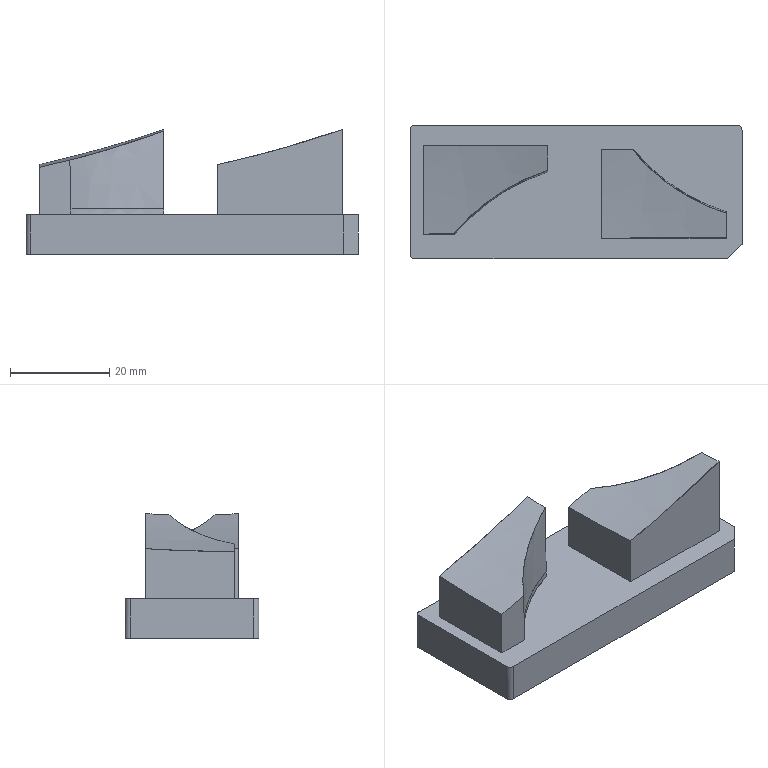NC program | PowerMill | posted with a generic post | part box 67 x 27 x 25.167 mm
Lines 24651 to 25366 of 102458:
N24748 M6
N24749 S18000 M03
N24750 G00 G90 X0.0 Y0.0
N24751 G43 Z10.797 H7
N24752
N24753 G05 P10000 R8
N24754 X29.8235 Y-9.0206
N24755 Z0.8472
N24756 G01 Z-0.3528 F1200.0
N24757 X29.7513 Y-9.0928 Z-0.3676 F2000.0
N24758 X29.6794 Y-9.1647 Z-0.3864
N24759 X29.5437 Y-9.2297 Z-0.4287
N24760 X29.5775 Y-9.1959 Z-0.419
N24761 X29.6113 Y-9.1621 Z-0.4095
N24762 X29.6452 Y-9.1282 Z-0.4002
N24763 X29.6932 Y-9.0802 Z-0.3873
N24764 X29.7271 Y-9.0463 Z-0.3787
N24765 X29.761 Y-9.0124 Z-0.3704
N24766 X29.795 Y-8.9784 Z-0.3627
N24767 X29.8292 Y-8.9442 Z-0.3563
N24768 X29.8343 Y-8.9391 Z-0.3555
N24769 X29.8422 Y-8.8605 Z-0.3588
N24770 X29.8358 Y-8.8669 Z-0.3597
N24771 X29.8102 Y-8.8925 Z-0.3643
N24772 X29.7846 Y-8.9181 Z-0.3698
N24773 X29.759 Y-8.9436 Z-0.3758
N24774 X29.7286 Y-8.9741 Z-0.3832
N24775 X29.6906 Y-9.0121 Z-0.3929
N24776 X29.6387 Y-9.064 Z-0.4066
N24777 X29.5843 Y-9.1184 Z-0.4214
N24778 X29.5453 Y-9.1574 Z-0.4322
N24779 X29.5143 Y-9.1884 Z-0.4409
N24780 X29.4888 Y-9.2139 Z-0.4481
N24781 X29.4634 Y-9.2393 Z-0.4553
N24782 X29.438 Y-9.2647 Z-0.4627
N24783 X29.3351 Y-9.2969 Z-0.4973
N24784 X29.4291 Y-9.2029 Z-0.469
N24785 X29.5517 Y-9.0802 Z-0.4354
N24786 X29.6657 Y-8.9663 Z-0.4042
N24787 X29.7395 Y-8.8924 Z-0.385
N24788 X29.7976 Y-8.8343 Z-0.3723
N24789 X29.8452 Y-8.7868 Z-0.3626
N24790 X29.8443 Y-8.717 Z-0.3677
N24791 X29.7502 Y-8.811 Z-0.3888
N24792 X29.6576 Y-8.9037 Z-0.4117
N24793 X29.5604 Y-9.0009 Z-0.438
N24794 X29.4297 Y-9.1315 Z-0.4726
N24795 X29.3322 Y-9.2291 Z-0.5005
N24796 X29.235 Y-9.3263 Z-0.5311
N24797 X29.1561 Y-9.3344 Z-0.5576
N24798 X29.2569 Y-9.2336 Z-0.526
N24799 X29.358 Y-9.1325 Z-0.4967
N24800 X29.481 Y-9.0095 Z-0.4642
N24801 X29.5915 Y-8.8991 Z-0.434
N24802 X29.683 Y-8.8076 Z-0.4092
N24803 X29.7582 Y-8.7324 Z-0.3914
N24804 X29.8436 Y-8.647 Z-0.373
N24805 X29.8432 Y-8.5766 Z-0.3777
N24806 X29.8386 Y-8.5812 Z-0.3787
N24807 X29.7357 Y-8.6842 Z-0.4013
N24808 X29.6434 Y-8.7765 Z-0.425
N24809 X29.5533 Y-8.8665 Z-0.4503
N24810 X29.3986 Y-9.0213 Z-0.4914
N24811 X29.3165 Y-9.1033 Z-0.5131
N24812 X29.2512 Y-9.1686 Z-0.5305
N24813 X29.1813 Y-9.2386 Z-0.5514
N24814 X29.0855 Y-9.3344 Z-0.5815
N24815 X29.0149 Y-9.3343 Z-0.6053
N24816 X29.1253 Y-9.2238 Z-0.5706
N24817 X29.2066 Y-9.1425 Z-0.5469
N24818 X29.3381 Y-9.0111 Z-0.5119
N24819 X29.4866 Y-8.8625 Z-0.4723
N24820 X29.6224 Y-8.7267 Z-0.4355
N24821 X29.7254 Y-8.6237 Z-0.4093
N24822 X29.8287 Y-8.5205 Z-0.3853
N24823 X29.8429 Y-8.5062 Z-0.3822
N24824 X29.8428 Y-8.4356 Z-0.3873
N24825 X29.8179 Y-8.4605 Z-0.3921
N24826 X29.7669 Y-8.5115 Z-0.4026
N24827 X29.7121 Y-8.5663 Z-0.4165
N24828 X29.6462 Y-8.6322 Z-0.4338
N24829 X29.5733 Y-8.7051 Z-0.4538
N24830 X29.4398 Y-8.8386 Z-0.4898
N24831 X29.2709 Y-9.0076 Z-0.5346
N24832 X29.1377 Y-9.1407 Z-0.5702
N24833 X29.0518 Y-9.2266 Z-0.5943
N24834 X28.9981 Y-9.2803 Z-0.6106
N24835 X28.9447 Y-9.3337 Z-0.6289
N24836 X28.8745 Y-9.3332 Z-0.6525
N24837 X28.9458 Y-9.2619 Z-0.6285
N24838 X29.0251 Y-9.1826 Z-0.6056
N24839 X29.1163 Y-9.0914 Z-0.5815
N24840 X29.4826 Y-8.7251 Z-0.4831
N24841 X29.5937 Y-8.614 Z-0.453
N24842 X29.6708 Y-8.5369 Z-0.4317
N24843 X29.7347 Y-8.473 Z-0.416
N24844 X29.8435 Y-8.3642 Z-0.3921
N24845 X29.8442 Y-8.2928 Z-0.3966
N24846 X29.7326 Y-8.4044 Z-0.4219
N24847 X29.6142 Y-8.5228 Z-0.4522
N24848 X29.3636 Y-8.7734 Z-0.52
N24849 X29.2147 Y-8.9223 Z-0.56
N24850 X29.0681 Y-9.0689 Z-0.5991
N24851 X28.9799 Y-9.1571 Z-0.6235
N24852 X28.8918 Y-9.2452 Z-0.6488
N24853 X28.8041 Y-9.3329 Z-0.6761
N24854 X28.7332 Y-9.3331 Z-0.6997
N24855 X28.8006 Y-9.2657 Z-0.677
N24856 X28.8781 Y-9.1882 Z-0.6547
N24857 X28.9737 Y-9.0926 Z-0.6293
N24858 X29.1969 Y-8.8694 Z-0.5697
N24859 X29.5364 Y-8.5299 Z-0.478
N24860 X29.5766 Y-8.4896 Z-0.4671
N24861 X29.6169 Y-8.4494 Z-0.4561
N24862 X29.6571 Y-8.4091 Z-0.4452
N24863 X29.6974 Y-8.3689 Z-0.4343
N24864 X29.7377 Y-8.3286 Z-0.4238
N24865 X29.7782 Y-8.2881 Z-0.4147
N24866 X29.8402 Y-8.2261 Z-0.4017
N24867 X29.8448 Y-8.2214 Z-0.4006
N24868 X29.8455 Y-8.1501 Z-0.4052
N24869 X29.7642 Y-8.2314 Z-0.4228
N24870 X29.6658 Y-8.3298 Z-0.4476
N24871 X29.3337 Y-8.6618 Z-0.5377
N24872 X29.0876 Y-8.908 Z-0.6034
N24873 X28.9239 Y-9.0717 Z-0.6473
N24874 X28.8365 Y-9.159 Z-0.6716
N24875 X28.7493 Y-9.2463 Z-0.6965
N24876 X28.6623 Y-9.3333 Z-0.7234
N24877 X28.5912 Y-9.3336 Z-0.747
N24878 X28.633 Y-9.2919 Z-0.7333
N24879 X28.6749 Y-9.25 Z-0.7203
N24880 X28.7169 Y-9.208 Z-0.7078
N24881 X28.7589 Y-9.1659 Z-0.6958
N24882 X28.8339 Y-9.091 Z-0.6763
N24883 X28.9115 Y-9.0134 Z-0.6555
N24884 X29.2718 Y-8.6531 Z-0.5592
N24885 X29.5281 Y-8.3967 Z-0.4897
N24886 X29.6897 Y-8.2351 Z-0.4456
N24887 X29.7662 Y-8.1586 Z-0.426
N24888 X29.8301 Y-8.0948 Z-0.4127
N24889 X29.8462 Y-8.0786 Z-0.4099
N24890 X29.8469 Y-8.0072 Z-0.4142
N24891 X29.8381 Y-8.0161 Z-0.4163
N24892 X29.7677 Y-8.0864 Z-0.4312
N24893 X29.7092 Y-8.145 Z-0.4447
N24894 X29.6195 Y-8.2347 Z-0.4689
N24895 X29.5075 Y-8.3467 Z-0.4999
N24896 X29.2882 Y-8.5659 Z-0.5588
N24897 X29.1348 Y-8.7193 Z-0.6008
N24898 X28.98 Y-8.8741 Z-0.6424
N24899 X28.8011 Y-9.0531 Z-0.6897
N24900 X28.7352 Y-9.1189 Z-0.7072
N24901 X28.675 Y-9.1791 Z-0.7231
N24902 X28.6084 Y-9.2457 Z-0.7429
N24903 X28.5201 Y-9.334 Z-0.7707
N24904 X28.449 Y-9.3344 Z-0.7944
N24905 X28.4996 Y-9.2838 Z-0.7778
N24906 X28.5504 Y-9.233 Z-0.7623
N24907 X28.6013 Y-9.1822 Z-0.7475
N24908 X28.6523 Y-9.1312 Z-0.7334
N24909 X28.7886 Y-8.9949 Z-0.6979
N24910 X28.9179 Y-8.8655 Z-0.6634
N24911 X29.2392 Y-8.5442 Z-0.5774
N24912 X29.5604 Y-8.2231 Z-0.4902
N24913 X29.6775 Y-8.106 Z-0.4586
N24914 X29.7922 Y-7.9912 Z-0.4304
N24915 X29.8475 Y-7.9359 Z-0.4182
N24916 X29.8482 Y-7.8645 Z-0.423
N24917 X29.8337 Y-7.8791 Z-0.426
N24918 X29.781 Y-7.9317 Z-0.4368
N24919 X29.7285 Y-7.9842 Z-0.4489
N24920 X29.6763 Y-8.0364 Z-0.463
N24921 X29.5794 Y-8.1333 Z-0.4897
N24922 X29.3857 Y-8.3271 Z-0.5425
N24923 X29.106 Y-8.6068 Z-0.618
N24924 X28.8903 Y-8.8224 Z-0.6759
N24925 X28.6646 Y-9.0481 Z-0.7356
N24926 X28.5943 Y-9.1184 Z-0.7542
N24927 X28.5337 Y-9.179 Z-0.7702
N24928 X28.4644 Y-9.2483 Z-0.7909
N24929 X28.3759 Y-9.3368 Z-0.8187
N24930 X28.3029 Y-9.3392 Z-0.843
N24931 X28.3967 Y-9.2453 Z-0.8136
N24932 X28.468 Y-9.1741 Z-0.7924
N24933 X28.5342 Y-9.1079 Z-0.7749
N24934 X28.6277 Y-9.0144 Z-0.7506
N24935 X29.0182 Y-8.6238 Z-0.6464
N24936 X29.3225 Y-8.3195 Z-0.5643
N24937 X29.6119 Y-8.0302 Z-0.4853
N24938 X29.7368 Y-7.9053 Z-0.4532
N24939 X29.8491 Y-7.793 Z-0.4276
N24940 X29.8498 Y-7.7215 Z-0.4318
N24941 X29.7512 Y-7.8201 Z-0.4538
N24942 X29.636 Y-7.9354 Z-0.4833
N24943 X29.4422 Y-8.1291 Z-0.5364
N24944 X29.0478 Y-8.5235 Z-0.6431
N24945 X28.5472 Y-9.0241 Z-0.7767
N24946 X28.4606 Y-9.1107 Z-0.7993
N24947 X28.3966 Y-9.1747 Z-0.8161
N24948 X28.3222 Y-9.2492 Z-0.8384
N24949 X28.2296 Y-9.3417 Z-0.8675
N24950 X28.156 Y-9.3446 Z-0.8919
N24951 X28.2525 Y-9.2481 Z-0.8617
N24952 X28.3296 Y-9.171 Z-0.8387
N24953 X28.3963 Y-9.1043 Z-0.8212
N24954 X28.4922 Y-9.0084 Z-0.7963
N24955 X28.7996 Y-8.701 Z-0.7141
N24956 X29.1069 Y-8.3937 Z-0.6315
N24957 X29.2847 Y-8.2159 Z-0.584
N24958 X29.4734 Y-8.0272 Z-0.5324
N24959 X29.6392 Y-7.8614 Z-0.4869
N24960 X29.7427 Y-7.7579 Z-0.4599
N24961 X29.8384 Y-7.6622 Z-0.4385
N24962 X29.8505 Y-7.6501 Z-0.436
N24963 X29.8514 Y-7.5785 Z-0.4408
N24964 X29.8415 Y-7.5884 Z-0.4425
N24965 X29.7692 Y-7.6607 Z-0.4571
N24966 X29.6939 Y-7.736 Z-0.4763
N24967 X29.5002 Y-7.9297 Z-0.5297
N24968 X29.0678 Y-8.362 Z-0.6472
N24969 X28.6342 Y-8.7957 Z-0.7633
N24970 X28.3958 Y-9.0341 Z-0.8263
N24971 X28.3207 Y-9.1092 Z-0.8461
N24972 X28.2581 Y-9.1718 Z-0.8625
N24973 X28.179 Y-9.2509 Z-0.886
N24974 X28.0825 Y-9.3474 Z-0.9164
N24975 X28.0118 Z-0.9398
N24976 X28.0841 Y-9.2751 Z-0.9155
N24977 X28.1662 Y-9.193 Z-0.8917
N24978 X28.2646 Y-9.0945 Z-0.8658
N24979 X28.6906 Y-8.6685 Z-0.7531
N24980 X29.1821 Y-8.1771 Z-0.6209
N24981 X29.5489 Y-7.8103 Z-0.5209
N24982 X29.6593 Y-7.6998 Z-0.4906
N24983 X29.7718 Y-7.5874 Z-0.4627
N24984 X29.8522 Y-7.507 Z-0.4451
N24985 X29.8523 Y-7.4362 Z-0.4489
N24986 X29.7637 Y-7.5248 Z-0.4688
N24987 X29.6542 Y-7.6343 Z-0.4967
N24988 X29.2417 Y-8.0468 Z-0.6093
N24989 X28.7211 Y-8.5674 Z-0.7497
N24990 X28.2003 Y-9.0882 Z-0.8876
N24991 X28.0962 Y-9.1923 Z-0.915
N24992 X28.0134 Y-9.275 Z-0.9389
N24993 X27.9418 Y-9.3466 Z-0.9628
N24994 X27.872 Y-9.3458 Z-0.9858
N24995 X27.9382 Y-9.2796 Z-0.9636
N24996 X28.0169 Y-9.2008 Z-0.9408
N24997 X28.125 Y-9.0928 Z-0.9123
N24998 X28.685 Y-8.5328 Z-0.7641
N24999 X29.0776 Y-8.1401 Z-0.6584
N25000 X29.3427 Y-7.8751 Z-0.5864
N25001 X29.5835 Y-7.6343 Z-0.5203
N25002 X29.6634 Y-7.5543 Z-0.4981
N25003 X29.7313 Y-7.4865 Z-0.4802
N25004 X29.7772 Y-7.4406 Z-0.4687
N25005 X29.8222 Y-7.3955 Z-0.4596
N25006 X29.8523 Y-7.3655 Z-0.4535
N25007 X29.8521 Y-7.2949 Z-0.4581
N25008 X29.8261 Y-7.321 Z-0.4626
N25009 X29.7785 Y-7.3685 Z-0.4728
N25010 X29.7312 Y-7.4159 Z-0.4845
N25011 X29.6839 Y-7.4632 Z-0.4967
N25012 X29.6087 Y-7.5384 Z-0.5178
N25013 X29.5308 Y-7.6163 Z-0.5393
N25014 X29.1435 Y-8.0035 Z-0.6451
N25015 X28.7131 Y-8.4339 Z-0.7613
N25016 X28.0517 Y-9.0953 Z-0.9364
N25017 X27.9456 Y-9.2015 Z-0.9643
N25018 X27.8682 Y-9.2789 Z-0.9866
N25019 X27.8031 Y-9.344 Z-1.0085
N25020 X27.7342 Y-9.3421 Z-1.0311
N25021 X27.7998 Y-9.2765 Z-1.0092
N25022 X27.8775 Y-9.1988 Z-0.9868
N25023 X27.9827 Y-9.0936 Z-0.9593
N25024 X28.4509 Y-8.6254 Z-0.8359
N25025 X29.0219 Y-8.0544 Z-0.6828
N25026 X29.4442 Y-7.6321 Z-0.5675
N25027 X29.6379 Y-7.4384 Z-0.5141
N25028 X29.7534 Y-7.323 Z-0.4844
N25029 X29.8504 Y-7.226 Z-0.4624
N25030 X29.8485 Y-7.1571 Z-0.4669
N25031 X29.7674 Y-7.2383 Z-0.4849
N25032 X29.6619 Y-7.3438 Z-0.5119
N25033 X29.4682 Y-7.5374 Z-0.5654
N25034 X29.1975 Y-7.8081 Z-0.6396
N25035 X28.8277 Y-8.1779 Z-0.7397
N25036 X28.2752 Y-8.7304 Z-0.8872
N25037 X27.9117 Y-9.0939 Z-0.9828
N25038 X27.8119 Y-9.1937 Z-1.0087
N25039 X27.7331 Y-9.2726 Z-1.0312
N25040 X27.665 Y-9.3406 Z-1.0539
N25041 X27.5952 Y-9.3398 Z-1.0769
N25042 X27.6613 Y-9.2737 Z-1.0548
N25043 X27.7393 Y-9.1956 Z-1.0325
N25044 X27.8434 Y-9.0915 Z-1.0055
N25045 X28.2051 Y-8.7298 Z-0.9105
N25046 X28.8205 Y-8.1145 Z-0.7464
N25047 X29.2506 Y-7.6843 Z-0.6294
N25048 X29.5661 Y-7.3688 Z-0.5426
N25049 X29.6492 Y-7.2857 Z-0.5192
N25050 X29.7124 Y-7.2226 Z-0.5025
N25051 X29.8078 Y-7.1271 Z-0.4806
N25052 X29.847 Y-7.0879 Z-0.4719
N25053 X29.8453 Y-7.0189 Z-0.4765
N25054 X29.7771 Y-7.0871 Z-0.4919
N25055 X29.654 Y-7.2102 Z-0.5228
N25056 X29.5314 Y-7.3328 Z-0.5566
N25057 X29.3567 Y-7.5075 Z-0.6048
N25058 X28.7894 Y-8.0749 Z-0.7593
N25059 X28.2216 Y-8.6426 Z-0.911
N25060 X27.7732 Y-9.091 Z-1.0286
N25061 X27.6688 Y-9.1954 Z-1.0557
N25062 X27.591 Y-9.2732 Z-1.078
N25063 X27.5253 Y-9.3389 Z-1.0999
N25064 X27.4552 Y-9.3383 Z-1.123
N25065 X27.5217 Y-9.2718 Z-1.1008
N25066 X27.5997 Y-9.1938 Z-1.0786
N25067 X27.702 Y-9.0915 Z-1.0521
N25068 X28.1852 Y-8.6083 Z-0.9254
N25069 X28.8038 Y-7.9897 Z-0.76
N25070 X29.4219 Y-7.3716 Z-0.5912
N25071 X29.6436 Y-7.1499 Z-0.53
N25072 X29.7523 Y-7.0412 Z-0.5018
N25073 X29.8435 Y-6.95 Z-0.4807
N25074 X29.8428 Y-6.88 Z-0.4855
N25075 X29.8409 Y-6.8819 Z-0.4858
N25076 X29.7987 Y-6.9241 Z-0.4939
N25077 X29.7567 Y-6.9661 Z-0.5038
N25078 X29.7149 Y-7.0079 Z-0.5149
N25079 X29.673 Y-7.0498 Z-0.526
N25080 X29.6299 Y-7.0929 Z-0.5378
N25081 X29.5552 Y-7.1676 Z-0.5586
N25082 X29.3825 Y-7.3402 Z-0.6065
N25083 X29.0187 Y-7.7041 Z-0.7063
N25084 X28.6324 Y-8.0904 Z-0.8107
N25085 X28.2444 Y-8.4784 Z-0.9144
N25086 X27.9727 Y-8.7501 Z-0.9863
N25087 X27.7009 Y-9.0219 Z-1.0571
N25088 X27.6213 Y-9.1015 Z-1.0778
N25089 X27.5558 Y-9.167 Z-1.0949
N25090 X27.484 Y-9.2388 Z-1.1157
N25091 X27.3848 Y-9.3379 Z-1.1461
N25092 X27.3145 Y-9.3376 Z-1.1693
N25093 X27.3462 Y-9.3058 Z-1.1592
N25094 X27.378 Y-9.274 Z-1.1495
N25095 X27.4134 Y-9.2386 Z-1.1389
N25096 X27.4453 Y-9.2068 Z-1.1295
N25097 X27.4771 Y-9.1749 Z-1.1203
N25098 X27.5091 Y-9.143 Z-1.1117
N25099 X27.5804 Y-9.0716 Z-1.0935
N25100 X27.8425 Y-8.8095 Z-1.0252
N25101 X28.1029 Y-8.5492 Z-0.9565
N25102 X28.5324 Y-8.1197 Z-0.8423
N25103 X28.9617 Y-7.6904 Z-0.7261
N25104 X29.2116 Y-7.4404 Z-0.6579
N25105 X29.4475 Y-7.2046 Z-0.5926
N25106 X29.5469 Y-7.1052 Z-0.5653
N25107 X29.6553 Y-6.9968 Z-0.5345
N25108 X29.7159 Y-6.9362 Z-0.5186
N25109 X29.7767 Y-6.8754 Z-0.5038
N25110 X29.8376 Y-6.8145 Z-0.4909
N25111 X29.8426 Y-6.8095 Z-0.49
N25112 X29.8423 Y-6.7391 Z-0.4941
N25113 X29.8397 Y-6.7416 Z-0.4948
N25114 X29.7749 Y-6.8065 Z-0.509
N25115 X29.718 Y-6.8633 Z-0.522
N25116 X29.6457 Y-6.9356 Z-0.5416
N25117 X29.54 Y-7.0414 Z-0.5716
N25118 X29.4444 Y-7.137 Z-0.5976
N25119 X29.2338 Y-7.3476 Z-0.6562
N25120 X28.8463 Y-7.7351 Z-0.762
N25121 X28.2852 Y-8.2961 Z-0.9128
N25122 X27.9516 Y-8.6297 Z-1.0013
N25123 X27.6179 Y-8.9635 Z-1.0885
N25124 X27.5077 Y-9.0737 Z-1.1169
N25125 X27.4164 Y-9.165 Z-1.1407
N25126 X27.3819 Y-9.1995 Z-1.1506
N25127 X27.3474 Y-9.234 Z-1.1607
N25128 X27.3129 Y-9.2684 Z-1.171
N25129 X27.2785 Y-9.3028 Z-1.1814
N25130 X27.2442 Y-9.3372 Z-1.1924
N25131 X27.1739 Y-9.3368 Z-1.2153
N25132 X27.241 Y-9.2697 Z-1.1932
N25133 X27.3202 Y-9.1904 Z-1.1708
N25134 X27.4263 Y-9.0843 Z-1.1433
N25135 X27.9594 Y-8.5512 Z-1.0039
N25136 X28.4631 Y-8.0476 Z-0.8698
N25137 X28.9664 Y-7.5443 Z-0.7335
N25138 X29.1954 Y-7.3152 Z-0.6711
N25139 X29.4473 Y-7.0633 Z-0.6015
N25140 X29.6134 Y-6.8973 Z-0.5553
N25141 X29.7319 Y-6.7788 Z-0.5238
N25142 X29.8356 Y-6.6751 Z-0.4993
N25143 X29.8418 Y-6.6689 Z-0.498
N25144 X29.8416 Y-6.5984 Z-0.5025
N25145 X29.8199 Y-6.62 Z-0.5071
N25146 X29.765 Y-6.6749 Z-0.519
N25147 X29.7103 Y-6.7296 Z-0.5326
N25148 X29.6558 Y-6.7841 Z-0.5478
N25149 X29.5733 Y-6.8666 Z-0.5709
N25150 X29.4327 Y-7.0072 Z-0.6099
N25151 X29.264 Y-7.176 Z-0.6567
N25152 X29.0952 Y-7.3448 Z-0.7029
N25153 X28.8271 Y-7.6128 Z-0.7756
N25154 X28.2777 Y-8.1622 Z-0.9241
N25155 X27.8204 Y-8.6196 Z-1.0452
N25156 X27.3568 Y-9.0832 Z-1.1662
N25157 X27.2511 Y-9.1889 Z-1.1935
N25158 X27.1713 Y-9.2686 Z-1.216
N25159 X27.1035 Y-9.3364 Z-1.2383
N25160 X27.0332 Y-9.336 Z-1.2612
N25161 X27.096 Y-9.2732 Z-1.2404
N25162 X27.172 Y-9.1972 Z-1.2189
N25163 X27.2839 Y-9.0854 Z-1.1899
N25164 X27.6963 Y-8.6729 Z-1.0826
N25165 X28.3443 Y-8.0249 Z-0.911
N25166 X28.6971 Y-7.6721 Z-0.8154
N25167 X29.0498 Y-7.3194 Z-0.7191
N25168 X29.3203 Y-7.0489 Z-0.6453
N25169 X29.631 Y-6.7382 Z-0.5589
N25170 X29.694 Y-6.6752 Z-0.5413
N25171 X29.7684 Y-6.6008 Z-0.5219
N25172 X29.8283 Y-6.5409 Z-0.5091
N25173 X29.8418 Y-6.5274 Z-0.5067
N25174 X29.8432 Y-6.4553 Z-0.5102
N25175 X29.7972 Y-6.5013 Z-0.5207
N25176 X29.6983 Y-6.6002 Z-0.5454
N25177 X29.5916 Y-6.7069 Z-0.5737
N25178 X29.4852 Y-6.8134 Z-0.6038
N25179 X29.3578 Y-6.9408 Z-0.639
N25180 X28.8575 Y-7.441 Z-0.7767
N25181 X28.2819 Y-8.0167 Z-0.9322
N25182 X27.8487 Y-8.4498 Z-1.0472
N25183 X27.5639 Y-8.7346 Z-1.1221
N25184 X27.2792 Y-9.0193 Z-1.1958
N25185 X27.1961 Y-9.1024 Z-1.2174
N25186 X27.1278 Y-9.1708 Z-1.235
N25187 X27.0608 Y-9.2377 Z-1.2543
N25188 X26.9629 Y-9.3356 Z-1.284
N25189 X26.8922 Z-1.307
N25190 X26.9619 Y-9.2659 Z-1.2841
N25191 X27.0404 Y-9.1875 Z-1.2623
N25192 X27.1326 Y-9.0952 Z-1.2387
N25193 X27.4516 Y-8.7762 Z-1.1561
N25194 X28.0826 Y-8.1452 Z-0.9899
N25195 X28.7762 Y-7.4516 Z-0.8033
N25196 X29.0694 Y-7.1584 Z-0.7226
N25197 X29.2645 Y-6.9633 Z-0.6693
N25198 X29.4145 Y-6.8134 Z-0.6275
N25199 X29.5549 Y-6.6729 Z-0.5885
N25200 X29.6309 Y-6.5969 Z-0.5672
N25201 X29.6951 Y-6.5327 Z-0.5494
N25202 X29.7489 Y-6.4789 Z-0.5348
N25203 X29.8032 Y-6.4247 Z-0.5228
N25204 X29.8445 Y-6.3833 Z-0.5136
N25205 X29.8461 Y-6.311 Z-0.5177
N25206 X29.8443 Y-6.3128 Z-0.5181
N25207 X29.7968 Y-6.3603 Z-0.5279
N25208 X29.7518 Y-6.4053 Z-0.5382
N25209 X29.6868 Y-6.4703 Z-0.5559
N25210 X29.6205 Y-6.5366 Z-0.5742
N25211 X29.5458 Y-6.6113 Z-0.5951
N25212 X29.3818 Y-6.7753 Z-0.641
N25213 X28.997 Y-7.1601 Z-0.7473
N25214 X28.5933 Y-7.5638 Z-0.8573
N25215 X27.9498 Y-8.2073 Z-1.0298
N25216 X27.3058 Y-8.8513 Z-1.1988
N25217 X27.0582 Y-9.0989 Z-1.2628
N25218 X26.9734 Y-9.1837 Z-1.2843
N25219 X26.8947 Y-9.2624 Z-1.3061
N25220 X26.8213 Y-9.3358 Z-1.3301
N25221 X26.7503 Y-9.3361 Z-1.3532
N25222 X26.8417 Y-9.2447 Z-1.3253
N25223 X26.9106 Y-9.1758 Z-1.3053
N25224 X26.9749 Y-9.1115 Z-1.2889
N25225 X27.0589 Y-9.0275 Z-1.2675
N25226 X27.5832 Y-8.5032 Z-1.1312
N25227 X28.1413 Y-7.9451 Z-0.9833
N25228 X28.6615 Y-7.4249 Z-0.8432
N25229 X29.2167 Y-6.8697 Z-0.691
N25230 X29.5701 Y-6.5163 Z-0.5926
N25231 X29.7007 Y-6.3857 Z-0.5556
N25232 X29.7734 Y-6.313 Z-0.5368
N25233 X29.8433 Y-6.243 Z-0.5225
N25234 X29.8476 Y-6.2388 Z-0.5217
N25235 X29.8491 Y-6.1666 Z-0.5254
N25236 X29.8448 Y-6.1708 Z-0.5264
N25237 X29.7809 Y-6.2348 Z-0.5403
N25238 X29.7251 Y-6.2906 Z-0.5531
N25239 X29.669 Y-6.3467 Z-0.5682
N25240 X29.5549 Y-6.4608 Z-0.6009
N25241 X29.4535 Y-6.5621 Z-0.629
N25242 X29.1443 Y-6.8714 Z-0.7152
N25243 X28.5228 Y-7.4929 Z-0.8852
N25244 X27.8837 Y-8.132 Z-1.0565
N25245 X27.2442 Y-8.7715 Z-1.2244
N25246 X26.9172 Y-9.0985 Z-1.3087
N25247 X26.8299 Y-9.1858 Z-1.3308
N25248 X26.7512 Y-9.2645 Z-1.3527
N25249 X26.679 Y-9.3367 Z-1.3764
N25250 X26.6076 Y-9.3374 Z-1.3997
N25251 X26.6791 Y-9.2659 Z-1.3761
N25252 X26.7576 Y-9.1874 Z-1.3542
N25253 X26.8457 Y-9.0993 Z-1.3319
N25254 X27.2271 Y-8.7178 Z-1.2336
N25255 X27.7256 Y-8.2194 Z-1.103
N25256 X28.4047 Y-7.5403 Z-0.9216
N25257 X29.0292 Y-6.9158 Z-0.7512
N25258 X29.6527 Y-6.2923 Z-0.5776
N25259 X29.7583 Y-6.1867 Z-0.55
N25260 X29.8505 Y-6.0945 Z-0.5287
N25261 X29.8519 Y-6.0223 Z-0.5329
N25262 X29.8391 Y-6.0351 Z-0.5355
N25263 X29.8105 Y-6.0638 Z-0.542
N25264 X29.7819 Y-6.0923 Z-0.5487
N25265 X29.7464 Y-6.1278 Z-0.5572
N25266 X29.7179 Y-6.1564 Z-0.5642
N25267 X29.6893 Y-6.1849 Z-0.5712
N25268 X29.6608 Y-6.2134 Z-0.5788
N25269 X29.5851 Y-6.2892 Z-0.6006
N25270 X29.1619 Y-6.7124 Z-0.7187
N25271 X28.4989 Y-7.3754 Z-0.9005
N25272 X27.8388 Y-8.0355 Z-1.0776
N25273 X27.1782 Y-8.6961 Z-1.2511
N25274 X26.7765 Y-9.0978 Z-1.3545
N25275 X26.6857 Y-9.1885 Z-1.3775
N25276 X26.6069 Y-9.2673 Z-1.3996
N25277 X26.5361 Y-9.3381 Z-1.4229
N25278 X26.4643 Y-9.3392 Z-1.4462
N25279 X26.5374 Y-9.2661 Z-1.4222
N25280 X26.6172 Y-9.1863 Z-1.4
N25281 X26.7058 Y-9.0978 Z-1.3775
N25282 X27.0453 Y-8.7582 Z-1.2903
N25283 X27.6898 Y-8.1137 Z-1.1217
N25284 X28.3273 Y-7.4763 Z-0.9513
N25285 X28.9643 Y-6.8392 Z-0.7775
N25286 X29.6008 Y-6.2027 Z-0.6002
N25287 X29.6764 Y-6.1271 Z-0.5783
N25288 X29.7328 Y-6.0708 Z-0.5638
N25289 X29.8213 Y-5.9822 Z-0.5439
N25290 X29.8533 Y-5.9502 Z-0.5368
N25291 X29.8545 Y-5.8784 Z-0.5404
N25292 X29.7511 Y-5.9817 Z-0.5639
N25293 X29.6406 Y-6.0923 Z-0.593
N25294 X29.427 Y-6.3059 Z-0.6531
N25295 X28.9898 Y-6.743 Z-0.7747
N25296 X28.5524 Y-7.1804 Z-0.8945
N25297 X28.0163 Y-7.7165 Z-1.0394
N25298 X27.4233 Y-8.3096 Z-1.1963
N25299 X26.8299 Y-8.903 Z-1.3507
N25300 X26.7037 Y-9.0292 Z-1.3824
N25301 X26.5819 Y-9.1509 Z-1.4135
N25302 X26.5344 Y-9.1984 Z-1.4265
N25303 X26.4869 Y-9.246 Z-1.4395
N25304 X26.4395 Y-9.2933 Z-1.4536
N25305 X26.3925 Y-9.3404 Z-1.4695
N25306 X26.3206 Y-9.3415 Z-1.4926
N25307 X26.388 Y-9.2741 Z-1.4705
N25308 X26.4673 Y-9.1948 Z-1.4482
N25309 X26.5717 Y-9.0904 Z-1.4216
N25310 X26.8389 Y-8.8233 Z-1.3531
N25311 X27.2589 Y-8.4032 Z-1.2441
N25312 X27.7157 Y-7.9464 Z-1.1241
N25313 X28.1722 Y-7.4899 Z-1.0018
N25314 X28.6384 Y-7.0237 Z-0.8753
N25315 X28.9491 Y-6.7131 Z-0.7903
N25316 X29.2804 Y-6.3817 Z-0.6981
N25317 X29.5194 Y-6.1427 Z-0.631
N25318 X29.6054 Y-6.0567 Z-0.6068
N25319 X29.6675 Y-5.9946 Z-0.5894
N25320 X29.7392 Y-5.923 Z-0.5698
N25321 X29.7924 Y-5.8698 Z-0.5571
N25322 X29.8516 Y-5.8105 Z-0.5446
N25323 X29.8554 Y-5.8067 Z-0.5437
N25324 X29.8542 Y-5.7372 Z-0.5482
N25325 X29.849 Y-5.7425 Z-0.5492
N25326 X29.8053 Y-5.7861 Z-0.5578
N25327 X29.7618 Y-5.8296 Z-0.5681
N25328 X29.7184 Y-5.873 Z-0.5795
N25329 X29.6751 Y-5.9163 Z-0.5909
N25330 X29.5967 Y-5.9947 Z-0.6132
N25331 X29.4032 Y-6.1882 Z-0.6678
N25332 X29.0652 Y-6.5262 Z-0.7621
N25333 X28.6094 Y-6.982 Z-0.8876
N25334 X28.0401 Y-7.5513 Z-1.0418
N25335 X27.604 Y-7.9874 Z-1.1582
N25336 X27.1486 Y-8.4428 Z-1.2776
N25337 X26.8562 Y-8.7353 Z-1.3535
N25338 X26.5636 Y-9.0278 Z-1.4283
N25339 X26.481 Y-9.1105 Z-1.4494
N25340 X26.4151 Y-9.1763 Z-1.4663
N25341 X26.3453 Y-9.2461 Z-1.4864
N25342 X26.2488 Y-9.3427 Z-1.5158
N25343 X26.1769 Y-9.3438 Z-1.5388
N25344 X26.242 Y-9.2787 Z-1.5174
N25345 X26.3193 Y-9.2014 Z-1.4957
N25346 X26.4253 Y-9.0955 Z-1.4686
N25347 X26.8977 Y-8.623 Z-1.3474
N25348 X27.37 Y-8.1507 Z-1.2244
N25349 X27.9605 Y-7.5602 Z-1.0675
N25350 X28.5506 Y-6.9701 Z-0.9079
N25351 X29.1178 Y-6.4029 Z-0.7516
N25352 X29.6269 Y-5.8939 Z-0.6087
N25353 X29.7422 Y-5.7785 Z-0.5781
N25354 X29.8521 Y-5.6686 Z-0.5524
N25355 X29.8499 Y-5.6001 Z-0.5562
N25356 X29.84 Y-5.61 Z-0.5583
N25357 X29.7453 Y-5.7047 Z-0.5811
N25358 X29.6508 Y-5.7992 Z-0.6059
N25359 X29.5214 Y-5.9286 Z-0.6419
N25360 X29.3609 Y-6.0891 Z-0.6877
N25361 X29.069 Y-6.381 Z-0.769
N25362 X28.5863 Y-6.8637 Z-0.9025
N25363 X28.0524 Y-7.3976 Z-1.0473
N25364 X27.3554 Y-8.0946 Z-1.2328
N25365 X27.031 Y-8.419 Z-1.3175
N25366 X26.6888 Y-8.7612 Z-1.4059
N25367 X26.5469 Y-8.9031 Z-1.4424
N25368 X26.4001 Y-9.0499 Z-1.4796
N25369 X26.3359 Y-9.1141 Z-1.4962
N25370 X26.2751 Y-9.1749 Z-1.5115
N25371 X26.2023 Y-9.2477 Z-1.5324
N25372 X26.1058 Y-9.3442 Z-1.5617
N25373 X26.0347 Y-9.3445 Z-1.5845
N25374 X26.13 Y-9.2493 Z-1.5556
N25375 X26.2039 Y-9.1754 Z-1.5344
N25376 X26.2694 Y-9.1099 Z-1.5178
N25377 X26.3571 Y-9.0222 Z-1.4957
N25378 X26.9238 Y-8.4555 Z-1.3501
N25379 X27.4901 Y-7.8892 Z-1.2018
N25380 X28.0801 Y-7.2992 Z-1.0443
N25381 X28.6932 Y-6.6861 Z-0.8773
N25382 X29.288 Y-6.0913 Z-0.7121
N25383 X29.5322 Y-5.8471 Z-0.6431
N25384 X29.6084 Y-5.7708 Z-0.6217
N25385 X29.6746 Y-5.7047 Z-0.603
N25386 X29.7408 Y-5.6385 Z-0.5847
N25387 X29.7854 Y-5.5939 Z-0.5737
N25388 X29.8385 Y-5.5408 Z-0.5628
N25389 X29.8478 Y-5.5315 Z-0.5607
N25390 X29.8457 Y-5.4628 Z-0.5651
N25391 X29.8424 Y-5.4662 Z-0.5657
N25392 X29.7741 Y-5.5344 Z-0.5799
N25393 X29.702 Y-5.6065 Z-0.5988
N25394 X29.5708 Y-5.7378 Z-0.6363
N25395 X29.2443 Y-6.0643 Z-0.7282
N25396 X28.7675 Y-6.5411 Z-0.861
N25397 X28.0588 Y-7.2498 Z-1.0543
N25398 X27.4468 Y-7.8618 Z-1.2178
N25399 X26.7687 Y-8.5399 Z-1.395
N25400 X26.2831 Y-9.0255 Z-1.5194
N25401 X26.2 Y-9.1086 Z-1.5403
N25402 X26.1352 Y-9.1734 Z-1.5566
N25403 X26.0597 Y-9.2488 Z-1.5782
N25404 X25.9638 Y-9.3447 Z-1.6073
N25405 X25.8934 Y-9.3445 Z-1.6299
N25406 X25.9873 Y-9.2506 Z-1.6015
N25407 X26.064 Y-9.1739 Z-1.5795
N25408 X26.1275 Y-9.1103 Z-1.5634
N25409 X26.2104 Y-9.0274 Z-1.5427
N25410 X26.8199 Y-8.418 Z-1.3865
N25411 X27.4289 Y-7.809 Z-1.227
N25412 X28.0859 Y-7.152 Z-1.0513
N25413 X28.7424 Y-6.4955 Z-0.8719
N25414 X29.0573 Y-6.1806 Z-0.7847
N25415 X29.3784 Y-5.8595 Z-0.6944
N25416 X29.5786 Y-5.6593 Z-0.6379
N25417 X29.7023 Y-5.5356 Z-0.6036
N25418 X29.8228 Y-5.4151 Z-0.5738
N25419 X29.8439 Y-5.394 Z-0.569
N25420 X29.843 Y-5.3241 Z-0.5728
N25421 X29.8163 Y-5.3508 Z-0.5788
N25422 X29.7126 Y-5.4546 Z-0.6043
N25423 X29.6032 Y-5.564 Z-0.6348
N25424 X29.4093 Y-5.7579 Z-0.6896
N25425 X29.1573 Y-6.0098 Z-0.7605
N25426 X28.6611 Y-6.506 Z-0.8986
N25427 X28.2582 Y-6.9089 Z-1.0088
N25428 X27.7401 Y-7.4271 Z-1.1487
N25429 X27.0639 Y-8.1033 Z-1.3275
N25430 X26.3872 Y-8.78 Z-1.5025
N25431 X26.0688 Y-9.0983 Z-1.5834
N25432 X25.9771 Y-9.1901 Z-1.6063
N25433 X25.8962 Y-9.2709 Z-1.6287
N25434 X25.823 Y-9.3442 Z-1.6525
N25435 X25.7526 Y-9.3439 Z-1.6752
N25436 X25.8239 Y-9.2726 Z-1.6526
N25437 X25.9175 Y-9.179 Z-1.6263
N25438 X25.9815 Y-9.1149 Z-1.61
N25439 X26.0656 Y-9.0308 Z-1.5891
N25440 X26.6133 Y-8.4831 Z-1.4491
N25441 X27.2766 Y-7.8199 Z-1.2762
N25442 X27.9465 Y-7.1499 Z-1.0975
N25443 X28.6204 Y-6.476 Z-0.9138
N25444 X28.9401 Y-6.1564 Z-0.825
N25445 X29.2597 Y-5.8368 Z-0.7356
N25446 X29.5792 Y-5.5173 Z-0.6455
N25447 X29.6796 Y-5.4169 Z-0.6166
N25448 X29.7272 Y-5.3693 Z-0.6031
N25449 X29.775 Y-5.3215 Z-0.5913
N25450 X29.823 Y-5.2734 Z-0.5811
N25451 X29.8424 Y-5.254 Z-0.5771
N25452 X29.8417 Y-5.184 Z-0.581
N25453 X29.7351 Y-5.2907 Z-0.6066
N25454 X29.6164 Y-5.4093 Z-0.6386
N25455 X29.2824 Y-5.7434 Z-0.7333
N25456 X28.81 Y-6.2157 Z-0.8654
N25457 X28.0942 Y-6.9316 Z-1.0618
N25458 X27.4467 Y-7.5791 Z-1.2357
N25459 X26.7774 Y-8.2483 Z-1.4114
N25460 X26.1769 Y-8.8488 Z-1.5657
N25461 X25.9272 Y-9.0985 Z-1.6289
N25462 X25.8399 Y-9.1859 Z-1.6506
N25463 X25.7584 Y-9.2673 Z-1.673